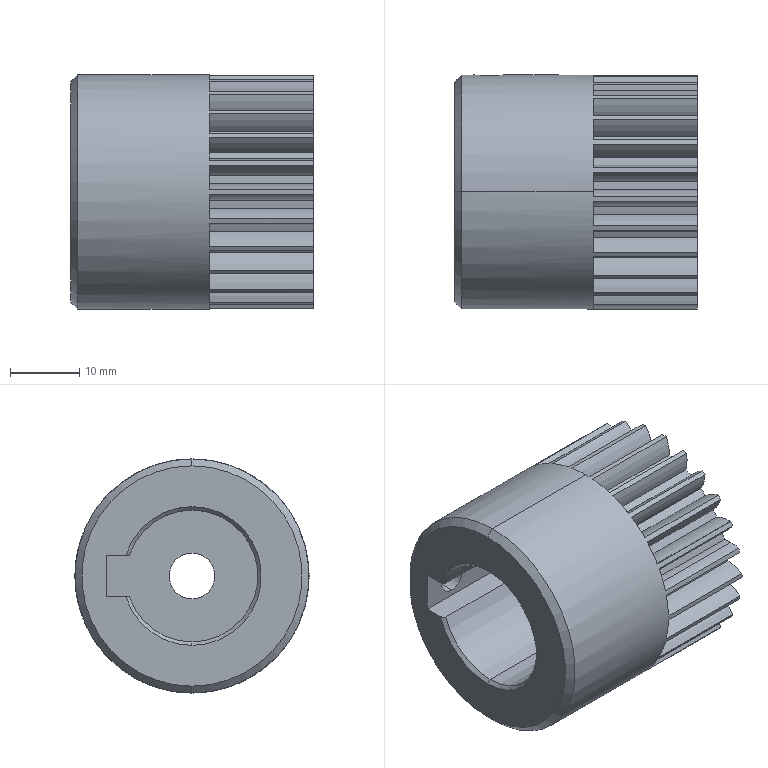Part | SolidWorks | features ICE 3, Chamfer 2, HoleWzd 2, BaseBody 1, MoveFace 1 | 1 solid | 127 faces | box 35 x 33.75 x 33.75 mm | volume 22032 mm3 | cylinder 90 | plane 32 | cone 5 | commonest cylinder face diameters 12.5 x54 28.123 x25 19 x3 4.2 x2 6.6 x2 11 x2